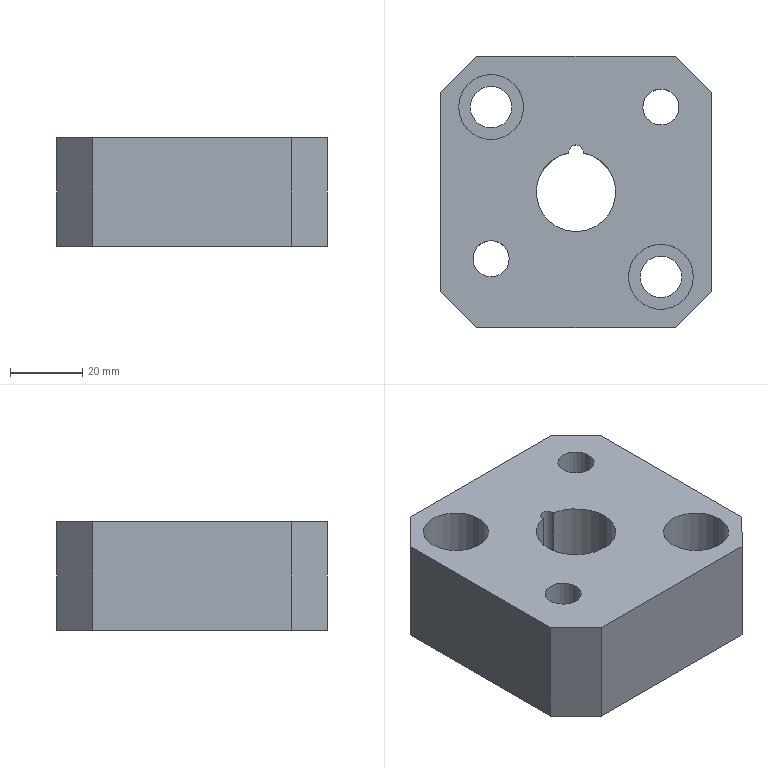Part | NX | features 23 2 | 1 solid | 20 faces | box 75 x 75 x 30 mm | volume 135687 mm3 | plane 12 | cylinder 8 | commonest cylinder face diameters 10.001 x2 11.5 x2 18 x2 4 x1 22 x1
STEP:
#1=CARTESIAN_POINT('',(23.298,10.818,-33.5));
#2=VERTEX_POINT('',#1);
#3=CARTESIAN_POINT('',(19.315,10.818,-33.5));
#4=VERTEX_POINT('',#3);
#5=CARTESIAN_POINT('',(21.306,11.,-33.5));
#6=DIRECTION('',(0.,0.,1.));
#7=DIRECTION('',(1.,0.,0.));
#8=AXIS2_PLACEMENT_3D('',#5,#6,#7);
#9=CIRCLE('',#8,2.);
#10=EDGE_CURVE('',#2,#4,#9,.T.);
#11=ORIENTED_EDGE('',*,*,#10,.T.);
#12=CARTESIAN_POINT('',(21.306,0.,-33.5));
#13=DIRECTION('',(0.,0.,-1.));
#14=DIRECTION('',(-1.,0.,0.));
#15=AXIS2_PLACEMENT_3D('',#12,#13,#14);
#16=CIRCLE('',#15,11.);
#17=EDGE_CURVE('',#2,#4,#16,.T.);
#18=ORIENTED_EDGE('',*,*,#17,.F.);
#19=EDGE_LOOP('',(#11,#18));
#20=FACE_BOUND('',#19,.T.);
#21=CARTESIAN_POINT('',(-7.194,-18.5,-33.5));
#22=VERTEX_POINT('',#21);
#23=CARTESIAN_POINT('',(-2.194,-18.5,-33.5));
#24=DIRECTION('',(0.,0.,-1.));
#25=DIRECTION('',(-1.,0.,0.));
#26=AXIS2_PLACEMENT_3D('',#23,#24,#25);
#27=CIRCLE('',#26,5.);
#28=EDGE_CURVE('',#22,#22,#27,.T.);
#29=ORIENTED_EDGE('',*,*,#28,.F.);
#30=EDGE_LOOP('',(#29));
#31=FACE_BOUND('',#30,.T.);
#32=CARTESIAN_POINT('',(-7.944,23.5,-33.5));
#33=VERTEX_POINT('',#32);
#34=CARTESIAN_POINT('',(-2.194,23.5,-33.5));
#35=DIRECTION('',(0.,0.,-1.));
#36=DIRECTION('',(-1.,0.,0.));
#37=AXIS2_PLACEMENT_3D('',#34,#35,#36);
#38=CIRCLE('',#37,5.75);
#39=EDGE_CURVE('',#33,#33,#38,.T.);
#40=ORIENTED_EDGE('',*,*,#39,.F.);
#41=EDGE_LOOP('',(#40));
#42=FACE_BOUND('',#41,.T.);
#43=CARTESIAN_POINT('',(39.806,23.5,-33.5));
#44=VERTEX_POINT('',#43);
#45=CARTESIAN_POINT('',(44.806,23.5,-33.5));
#46=DIRECTION('',(0.,0.,-1.));
#47=DIRECTION('',(-1.,0.,0.));
#48=AXIS2_PLACEMENT_3D('',#45,#46,#47);
#49=CIRCLE('',#48,5.);
#50=EDGE_CURVE('',#44,#44,#49,.T.);
#51=ORIENTED_EDGE('',*,*,#50,.F.);
#52=EDGE_LOOP('',(#51));
#53=FACE_BOUND('',#52,.T.);
#54=CARTESIAN_POINT('',(39.056,-23.5,-33.5));
#55=VERTEX_POINT('',#54);
#56=CARTESIAN_POINT('',(44.806,-23.5,-33.5));
#57=DIRECTION('',(0.,0.,-1.));
#58=DIRECTION('',(-1.,0.,0.));
#59=AXIS2_PLACEMENT_3D('',#56,#57,#58);
#60=CIRCLE('',#59,5.75);
#61=EDGE_CURVE('',#55,#55,#60,.T.);
#62=ORIENTED_EDGE('',*,*,#61,.F.);
#63=EDGE_LOOP('',(#62));
#64=FACE_BOUND('',#63,.T.);
#65=CARTESIAN_POINT('',(58.806,-27.5,-33.5));
#66=VERTEX_POINT('',#65);
#67=CARTESIAN_POINT('',(58.806,27.5,-33.5));
#68=VERTEX_POINT('',#67);
#69=CARTESIAN_POINT('',(58.806,0.,-33.5));
#70=DIRECTION('',(0.,1.,0.));
#71=VECTOR('',#70,1000.);
#72=LINE('',#69,#71);
#73=EDGE_CURVE('',#66,#68,#72,.T.);
#74=ORIENTED_EDGE('',*,*,#73,.F.);
#75=CARTESIAN_POINT('',(48.806,-37.5,-33.5));
#76=VERTEX_POINT('',#75);
#77=CARTESIAN_POINT('',(55.297,-31.009,-33.5));
#78=DIRECTION('',(-0.7071,-0.7071,0.));
#79=VECTOR('',#78,1000.);
#80=LINE('',#77,#79);
#81=EDGE_CURVE('',#66,#76,#80,.T.);
#82=ORIENTED_EDGE('',*,*,#81,.T.);
#83=CARTESIAN_POINT('',(-6.194,-37.5,-33.5));
#84=VERTEX_POINT('',#83);
#85=CARTESIAN_POINT('',(21.306,-37.5,-33.5));
#86=DIRECTION('',(1.,0.,0.));
#87=VECTOR('',#86,1000.);
#88=LINE('',#85,#87);
#89=EDGE_CURVE('',#84,#76,#88,.T.);
#90=ORIENTED_EDGE('',*,*,#89,.F.);
#91=CARTESIAN_POINT('',(-16.194,-27.5,-33.5));
#92=VERTEX_POINT('',#91);
#93=CARTESIAN_POINT('',(19.741,-63.435,-33.5));
#94=DIRECTION('',(-0.7071,0.7071,0.));
#95=VECTOR('',#94,1000.);
#96=LINE('',#93,#95);
#97=EDGE_CURVE('',#84,#92,#96,.T.);
#98=ORIENTED_EDGE('',*,*,#97,.T.);
#99=CARTESIAN_POINT('',(-16.194,27.5,-33.5));
#100=VERTEX_POINT('',#99);
#101=CARTESIAN_POINT('',(-16.194,0.,-33.5));
#102=DIRECTION('',(0.,-1.,0.));
#103=VECTOR('',#102,1000.);
#104=LINE('',#101,#103);
#105=EDGE_CURVE('',#100,#92,#104,.T.);
#106=ORIENTED_EDGE('',*,*,#105,.F.);
#107=CARTESIAN_POINT('',(-6.194,37.5,-33.5));
#108=VERTEX_POINT('',#107);
#109=CARTESIAN_POINT('',(-14.703,28.991,-33.5));
#110=DIRECTION('',(0.7071,0.7071,0.));
#111=VECTOR('',#110,1000.);
#112=LINE('',#109,#111);
#113=EDGE_CURVE('',#100,#108,#112,.T.);
#114=ORIENTED_EDGE('',*,*,#113,.T.);
#115=CARTESIAN_POINT('',(48.806,37.5,-33.5));
#116=VERTEX_POINT('',#115);
#117=CARTESIAN_POINT('',(21.306,37.5,-33.5));
#118=DIRECTION('',(-1.,0.,0.));
#119=VECTOR('',#118,1000.);
#120=LINE('',#117,#119);
#121=EDGE_CURVE('',#116,#108,#120,.T.);
#122=ORIENTED_EDGE('',*,*,#121,.F.);
#123=CARTESIAN_POINT('',(89.741,-3.435,-33.5));
#124=DIRECTION('',(0.7071,-0.7071,0.));
#125=VECTOR('',#124,1000.);
#126=LINE('',#123,#125);
#127=EDGE_CURVE('',#116,#68,#126,.T.);
#128=ORIENTED_EDGE('',*,*,#127,.T.);
#129=EDGE_LOOP('',(#74,#82,#90,#98,#106,#114,#122,#128));
#130=FACE_BOUND('',#129,.T.);
#131=CARTESIAN_POINT('',(53.733,-34.444,-33.5));
#132=DIRECTION('',(0.,0.,-1.));
#133=DIRECTION('',(-1.,0.,0.));
#134=AXIS2_PLACEMENT_3D('',#131,#132,#133);
#135=PLANE('',#134);
#136=ADVANCED_FACE('',(#20,#31,#42,#53,#64,#130),#135,.T.);
#137=CARTESIAN_POINT('',(19.315,10.818,-3.5));
#138=VERTEX_POINT('',#137);
#139=CARTESIAN_POINT('',(23.298,10.818,-3.5));
#140=VERTEX_POINT('',#139);
#141=CARTESIAN_POINT('',(21.306,0.,-3.5));
#142=DIRECTION('',(0.,0.,1.));
#143=DIRECTION('',(-1.,0.,0.));
#144=AXIS2_PLACEMENT_3D('',#141,#142,#143);
#145=CIRCLE('',#144,11.);
#146=EDGE_CURVE('',#138,#140,#145,.T.);
#147=ORIENTED_EDGE('',*,*,#146,.F.);
#148=CARTESIAN_POINT('',(21.306,11.,-3.5));
#149=DIRECTION('',(0.,0.,-1.));
#150=DIRECTION('',(-1.,0.,0.));
#151=AXIS2_PLACEMENT_3D('',#148,#149,#150);
#152=CIRCLE('',#151,2.);
#153=EDGE_CURVE('',#138,#140,#152,.T.);
#154=ORIENTED_EDGE('',*,*,#153,.T.);
#155=EDGE_LOOP('',(#147,#154));
#156=FACE_BOUND('',#155,.T.);
#157=CARTESIAN_POINT('',(-11.194,23.5,-3.5));
#158=VERTEX_POINT('',#157);
#159=CARTESIAN_POINT('',(-2.194,23.5,-3.5));
#160=DIRECTION('',(0.,0.,-1.));
#161=DIRECTION('',(-1.,0.,0.));
#162=AXIS2_PLACEMENT_3D('',#159,#160,#161);
#163=CIRCLE('',#162,9.);
#164=EDGE_CURVE('',#158,#158,#163,.T.);
#165=ORIENTED_EDGE('',*,*,#164,.T.);
#166=EDGE_LOOP('',(#165));
#167=FACE_BOUND('',#166,.T.);
#168=CARTESIAN_POINT('',(39.806,23.5,-3.5));
#169=VERTEX_POINT('',#168);
#170=CARTESIAN_POINT('',(44.806,23.5,-3.5));
#171=DIRECTION('',(0.,0.,1.));
#172=DIRECTION('',(-1.,0.,0.));
#173=AXIS2_PLACEMENT_3D('',#170,#171,#172);
#174=CIRCLE('',#173,5.);
#175=EDGE_CURVE('',#169,#169,#174,.T.);
#176=ORIENTED_EDGE('',*,*,#175,.F.);
#177=EDGE_LOOP('',(#176));
#178=FACE_BOUND('',#177,.T.);
#179=CARTESIAN_POINT('',(48.806,-37.5,-3.5));
#180=VERTEX_POINT('',#179);
#181=CARTESIAN_POINT('',(-6.194,-37.5,-3.5));
#182=VERTEX_POINT('',#181);
#183=CARTESIAN_POINT('',(21.306,-37.5,-3.5));
#184=DIRECTION('',(-1.,0.,0.));
#185=VECTOR('',#184,1000.);
#186=LINE('',#183,#185);
#187=EDGE_CURVE('',#180,#182,#186,.T.);
#188=ORIENTED_EDGE('',*,*,#187,.F.);
#189=CARTESIAN_POINT('',(58.806,-27.5,-3.5));
#190=VERTEX_POINT('',#189);
#191=CARTESIAN_POINT('',(64.18,-22.126,-3.5));
#192=DIRECTION('',(0.7071,0.7071,0.));
#193=VECTOR('',#192,1000.);
#194=LINE('',#191,#193);
#195=EDGE_CURVE('',#180,#190,#194,.T.);
#196=ORIENTED_EDGE('',*,*,#195,.T.);
#197=CARTESIAN_POINT('',(58.806,27.5,-3.5));
#198=VERTEX_POINT('',#197);
#199=CARTESIAN_POINT('',(58.806,0.,-3.5));
#200=DIRECTION('',(0.,-1.,0.));
#201=VECTOR('',#200,1000.);
#202=LINE('',#199,#201);
#203=EDGE_CURVE('',#198,#190,#202,.T.);
#204=ORIENTED_EDGE('',*,*,#203,.F.);
#205=CARTESIAN_POINT('',(48.806,37.5,-3.5));
#206=VERTEX_POINT('',#205);
#207=CARTESIAN_POINT('',(41.505,44.802,-3.5));
#208=DIRECTION('',(-0.7071,0.7071,0.));
#209=VECTOR('',#208,1000.);
#210=LINE('',#207,#209);
#211=EDGE_CURVE('',#198,#206,#210,.T.);
#212=ORIENTED_EDGE('',*,*,#211,.T.);
#213=CARTESIAN_POINT('',(-6.194,37.5,-3.5));
#214=VERTEX_POINT('',#213);
#215=CARTESIAN_POINT('',(21.306,37.5,-3.5));
#216=DIRECTION('',(1.,0.,0.));
#217=VECTOR('',#216,1000.);
#218=LINE('',#215,#217);
#219=EDGE_CURVE('',#214,#206,#218,.T.);
#220=ORIENTED_EDGE('',*,*,#219,.F.);
#221=CARTESIAN_POINT('',(-16.194,27.5,-3.5));
#222=VERTEX_POINT('',#221);
#223=CARTESIAN_POINT('',(-5.82,37.874,-3.5));
#224=DIRECTION('',(-0.7071,-0.7071,0.));
#225=VECTOR('',#224,1000.);
#226=LINE('',#223,#225);
#227=EDGE_CURVE('',#214,#222,#226,.T.);
#228=ORIENTED_EDGE('',*,*,#227,.T.);
#229=CARTESIAN_POINT('',(-16.194,-27.5,-3.5));
#230=VERTEX_POINT('',#229);
#231=CARTESIAN_POINT('',(-16.194,0.,-3.5));
#232=DIRECTION('',(0.,1.,0.));
#233=VECTOR('',#232,1000.);
#234=LINE('',#231,#233);
#235=EDGE_CURVE('',#230,#222,#234,.T.);
#236=ORIENTED_EDGE('',*,*,#235,.F.);
#237=CARTESIAN_POINT('',(-28.495,-15.198,-3.5));
#238=DIRECTION('',(0.7071,-0.7071,0.));
#239=VECTOR('',#238,1000.);
#240=LINE('',#237,#239);
#241=EDGE_CURVE('',#230,#182,#240,.T.);
#242=ORIENTED_EDGE('',*,*,#241,.T.);
#243=EDGE_LOOP('',(#188,#196,#204,#212,#220,#228,#236,#242));
#244=FACE_BOUND('',#243,.T.);
#245=CARTESIAN_POINT('',(35.806,-23.5,-3.5));
#246=VERTEX_POINT('',#245);
#247=CARTESIAN_POINT('',(44.806,-23.5,-3.5));
#248=DIRECTION('',(0.,0.,-1.));
#249=DIRECTION('',(-1.,0.,0.));
#250=AXIS2_PLACEMENT_3D('',#247,#248,#249);
#251=CIRCLE('',#250,9.);
#252=EDGE_CURVE('',#246,#246,#251,.T.);
#253=ORIENTED_EDGE('',*,*,#252,.T.);
#254=EDGE_LOOP('',(#253));
#255=FACE_BOUND('',#254,.T.);
#256=CARTESIAN_POINT('',(-7.194,-18.5,-3.5));
#257=VERTEX_POINT('',#256);
#258=CARTESIAN_POINT('',(-2.194,-18.5,-3.5));
#259=DIRECTION('',(0.,0.,1.));
#260=DIRECTION('',(-1.,0.,0.));
#261=AXIS2_PLACEMENT_3D('',#258,#259,#260);
#262=CIRCLE('',#261,5.);
#263=EDGE_CURVE('',#257,#257,#262,.T.);
#264=ORIENTED_EDGE('',*,*,#263,.F.);
#265=EDGE_LOOP('',(#264));
#266=FACE_BOUND('',#265,.T.);
#267=CARTESIAN_POINT('',(14.378,22.675,-3.5));
#268=DIRECTION('',(0.,0.,-1.));
#269=DIRECTION('',(-1.,0.,0.));
#270=AXIS2_PLACEMENT_3D('',#267,#268,#269);
#271=PLANE('',#270);
#272=ADVANCED_FACE('',(#156,#167,#178,#244,#255,#266),#271,.F.);
#273=ORIENTED_EDGE('',*,*,#89,.T.);
#274=CARTESIAN_POINT('',(48.806,-37.5,-23.5));
#275=DIRECTION('',(0.,0.,1.));
#276=VECTOR('',#275,1000.);
#277=LINE('',#274,#276);
#278=EDGE_CURVE('',#76,#180,#277,.T.);
#279=ORIENTED_EDGE('',*,*,#278,.T.);
#280=ORIENTED_EDGE('',*,*,#187,.T.);
#281=CARTESIAN_POINT('',(-6.194,-37.5,-23.5));
#282=DIRECTION('',(0.,0.,-1.));
#283=VECTOR('',#282,1000.);
#284=LINE('',#281,#283);
#285=EDGE_CURVE('',#182,#84,#284,.T.);
#286=ORIENTED_EDGE('',*,*,#285,.T.);
#287=EDGE_LOOP('',(#273,#279,#280,#286));
#288=FACE_BOUND('',#287,.T.);
#289=CARTESIAN_POINT('',(21.306,-37.5,-23.5));
#290=DIRECTION('',(0.,-1.,0.));
#291=DIRECTION('',(0.,0.,-1.));
#292=AXIS2_PLACEMENT_3D('',#289,#290,#291);
#293=PLANE('',#292);
#294=ADVANCED_FACE('',(#288),#293,.T.);
#295=ORIENTED_EDGE('',*,*,#235,.T.);
#296=CARTESIAN_POINT('',(-16.194,27.5,-23.5));
#297=DIRECTION('',(0.,0.,-1.));
#298=VECTOR('',#297,1000.);
#299=LINE('',#296,#298);
#300=EDGE_CURVE('',#222,#100,#299,.T.);
#301=ORIENTED_EDGE('',*,*,#300,.T.);
#302=ORIENTED_EDGE('',*,*,#105,.T.);
#303=CARTESIAN_POINT('',(-16.194,-27.5,-23.5));
#304=DIRECTION('',(0.,0.,1.));
#305=VECTOR('',#304,1000.);
#306=LINE('',#303,#305);
#307=EDGE_CURVE('',#92,#230,#306,.T.);
#308=ORIENTED_EDGE('',*,*,#307,.T.);
#309=EDGE_LOOP('',(#295,#301,#302,#308));
#310=FACE_BOUND('',#309,.T.);
#311=CARTESIAN_POINT('',(-16.194,0.,-23.5));
#312=DIRECTION('',(-1.,0.,0.));
#313=DIRECTION('',(0.,0.,1.));
#314=AXIS2_PLACEMENT_3D('',#311,#312,#313);
#315=PLANE('',#314);
#316=ADVANCED_FACE('',(#310),#315,.T.);
#317=ORIENTED_EDGE('',*,*,#219,.T.);
#318=CARTESIAN_POINT('',(48.806,37.5,-23.5));
#319=DIRECTION('',(0.,0.,-1.));
#320=VECTOR('',#319,1000.);
#321=LINE('',#318,#320);
#322=EDGE_CURVE('',#206,#116,#321,.T.);
#323=ORIENTED_EDGE('',*,*,#322,.T.);
#324=ORIENTED_EDGE('',*,*,#121,.T.);
#325=CARTESIAN_POINT('',(-6.194,37.5,-23.5));
#326=DIRECTION('',(0.,0.,1.));
#327=VECTOR('',#326,1000.);
#328=LINE('',#325,#327);
#329=EDGE_CURVE('',#108,#214,#328,.T.);
#330=ORIENTED_EDGE('',*,*,#329,.T.);
#331=EDGE_LOOP('',(#317,#323,#324,#330));
#332=FACE_BOUND('',#331,.T.);
#333=CARTESIAN_POINT('',(21.306,37.5,-23.5));
#334=DIRECTION('',(0.,1.,0.));
#335=DIRECTION('',(0.,0.,1.));
#336=AXIS2_PLACEMENT_3D('',#333,#334,#335);
#337=PLANE('',#336);
#338=ADVANCED_FACE('',(#332),#337,.T.);
#339=ORIENTED_EDGE('',*,*,#203,.T.);
#340=CARTESIAN_POINT('',(58.806,-27.5,-23.5));
#341=DIRECTION('',(0.,0.,-1.));
#342=VECTOR('',#341,1000.);
#343=LINE('',#340,#342);
#344=EDGE_CURVE('',#190,#66,#343,.T.);
#345=ORIENTED_EDGE('',*,*,#344,.T.);
#346=ORIENTED_EDGE('',*,*,#73,.T.);
#347=CARTESIAN_POINT('',(58.806,27.5,-23.5));
#348=DIRECTION('',(0.,0.,1.));
#349=VECTOR('',#348,1000.);
#350=LINE('',#347,#349);
#351=EDGE_CURVE('',#68,#198,#350,.T.);
#352=ORIENTED_EDGE('',*,*,#351,.T.);
#353=EDGE_LOOP('',(#339,#345,#346,#352));
#354=FACE_BOUND('',#353,.T.);
#355=CARTESIAN_POINT('',(58.806,0.,-23.5));
#356=DIRECTION('',(1.,0.,0.));
#357=DIRECTION('',(0.,0.,-1.));
#358=AXIS2_PLACEMENT_3D('',#355,#356,#357);
#359=PLANE('',#358);
#360=ADVANCED_FACE('',(#354),#359,.T.);
#361=ORIENTED_EDGE('',*,*,#61,.T.);
#362=EDGE_LOOP('',(#361));
#363=FACE_BOUND('',#362,.T.);
#364=CARTESIAN_POINT('',(39.056,-23.5,-18.5));
#365=VERTEX_POINT('',#364);
#366=CARTESIAN_POINT('',(44.806,-23.5,-18.5));
#367=DIRECTION('',(0.,0.,-1.));
#368=DIRECTION('',(-1.,0.,0.));
#369=AXIS2_PLACEMENT_3D('',#366,#367,#368);
#370=CIRCLE('',#369,5.75);
#371=EDGE_CURVE('',#365,#365,#370,.T.);
#372=ORIENTED_EDGE('',*,*,#371,.F.);
#373=EDGE_LOOP('',(#372));
#374=FACE_BOUND('',#373,.T.);
#375=CARTESIAN_POINT('',(44.806,-23.5,-1.5));
#376=DIRECTION('',(0.,0.,-1.));
#377=DIRECTION('',(1.,0.,0.));
#378=AXIS2_PLACEMENT_3D('',#375,#376,#377);
#379=CYLINDRICAL_SURFACE('',#378,5.75);
#380=ADVANCED_FACE('',(#363,#374),#379,.F.);
#381=ORIENTED_EDGE('',*,*,#371,.T.);
#382=EDGE_LOOP('',(#381));
#383=FACE_BOUND('',#382,.T.);
#384=CARTESIAN_POINT('',(35.806,-23.5,-18.5));
#385=VERTEX_POINT('',#384);
#386=CARTESIAN_POINT('',(44.806,-23.5,-18.5));
#387=DIRECTION('',(0.,0.,-1.));
#388=DIRECTION('',(-1.,0.,0.));
#389=AXIS2_PLACEMENT_3D('',#386,#387,#388);
#390=CIRCLE('',#389,9.);
#391=EDGE_CURVE('',#385,#385,#390,.T.);
#392=ORIENTED_EDGE('',*,*,#391,.F.);
#393=EDGE_LOOP('',(#392));
#394=FACE_BOUND('',#393,.T.);
#395=CARTESIAN_POINT('',(44.806,-23.5,-18.5));
#396=DIRECTION('',(0.,0.,-1.));
#397=DIRECTION('',(-1.,0.,0.));
#398=AXIS2_PLACEMENT_3D('',#395,#396,#397);
#399=PLANE('',#398);
#400=ADVANCED_FACE('',(#383,#394),#399,.F.);
#401=ORIENTED_EDGE('',*,*,#391,.T.);
#402=EDGE_LOOP('',(#401));
#403=FACE_BOUND('',#402,.T.);
#404=ORIENTED_EDGE('',*,*,#252,.F.);
#405=EDGE_LOOP('',(#404));
#406=FACE_BOUND('',#405,.T.);
#407=CARTESIAN_POINT('',(44.806,-23.5,-3.5));
#408=DIRECTION('',(0.,0.,-1.));
#409=DIRECTION('',(1.,0.,0.));
#410=AXIS2_PLACEMENT_3D('',#407,#408,#409);
#411=CYLINDRICAL_SURFACE('',#410,9.);
#412=ADVANCED_FACE('',(#403,#406),#411,.F.);
#413=ORIENTED_EDGE('',*,*,#175,.T.);
#414=EDGE_LOOP('',(#413));
#415=FACE_BOUND('',#414,.T.);
#416=ORIENTED_EDGE('',*,*,#50,.T.);
#417=EDGE_LOOP('',(#416));
#418=FACE_BOUND('',#417,.T.);
#419=CARTESIAN_POINT('',(44.806,23.5,198.5));
#420=DIRECTION('',(0.,0.,-1.));
#421=DIRECTION('',(-1.,0.,0.));
#422=AXIS2_PLACEMENT_3D('',#419,#420,#421);
#423=CYLINDRICAL_SURFACE('',#422,5.);
#424=ADVANCED_FACE('',(#415,#418),#423,.F.);
#425=ORIENTED_EDGE('',*,*,#39,.T.);
#426=EDGE_LOOP('',(#425));
#427=FACE_BOUND('',#426,.T.);
#428=CARTESIAN_POINT('',(-7.944,23.5,-18.5));
#429=VERTEX_POINT('',#428);
#430=CARTESIAN_POINT('',(-2.194,23.5,-18.5));
#431=DIRECTION('',(0.,0.,-1.));
#432=DIRECTION('',(-1.,0.,0.));
#433=AXIS2_PLACEMENT_3D('',#430,#431,#432);
#434=CIRCLE('',#433,5.75);
#435=EDGE_CURVE('',#429,#429,#434,.T.);
#436=ORIENTED_EDGE('',*,*,#435,.F.);
#437=EDGE_LOOP('',(#436));
#438=FACE_BOUND('',#437,.T.);
#439=CARTESIAN_POINT('',(-2.194,23.5,-1.5));
#440=DIRECTION('',(0.,0.,-1.));
#441=DIRECTION('',(1.,0.,0.));
#442=AXIS2_PLACEMENT_3D('',#439,#440,#441);
#443=CYLINDRICAL_SURFACE('',#442,5.75);
#444=ADVANCED_FACE('',(#427,#438),#443,.F.);
#445=ORIENTED_EDGE('',*,*,#435,.T.);
#446=EDGE_LOOP('',(#445));
#447=FACE_BOUND('',#446,.T.);
#448=CARTESIAN_POINT('',(-11.194,23.5,-18.5));
#449=VERTEX_POINT('',#448);
#450=CARTESIAN_POINT('',(-2.194,23.5,-18.5));
#451=DIRECTION('',(0.,0.,-1.));
#452=DIRECTION('',(-1.,0.,0.));
#453=AXIS2_PLACEMENT_3D('',#450,#451,#452);
#454=CIRCLE('',#453,9.);
#455=EDGE_CURVE('',#449,#449,#454,.T.);
#456=ORIENTED_EDGE('',*,*,#455,.F.);
#457=EDGE_LOOP('',(#456));
#458=FACE_BOUND('',#457,.T.);
#459=CARTESIAN_POINT('',(-2.194,23.5,-18.5));
#460=DIRECTION('',(0.,0.,-1.));
#461=DIRECTION('',(-1.,0.,0.));
#462=AXIS2_PLACEMENT_3D('',#459,#460,#461);
#463=PLANE('',#462);
#464=ADVANCED_FACE('',(#447,#458),#463,.F.);
#465=ORIENTED_EDGE('',*,*,#455,.T.);
#466=EDGE_LOOP('',(#465));
#467=FACE_BOUND('',#466,.T.);
#468=ORIENTED_EDGE('',*,*,#164,.F.);
#469=EDGE_LOOP('',(#468));
#470=FACE_BOUND('',#469,.T.);
#471=CARTESIAN_POINT('',(-2.194,23.5,-3.5));
#472=DIRECTION('',(0.,0.,-1.));
#473=DIRECTION('',(1.,0.,0.));
#474=AXIS2_PLACEMENT_3D('',#471,#472,#473);
#475=CYLINDRICAL_SURFACE('',#474,9.);
#476=ADVANCED_FACE('',(#467,#470),#475,.F.);
#477=ORIENTED_EDGE('',*,*,#263,.T.);
#478=EDGE_LOOP('',(#477));
#479=FACE_BOUND('',#478,.T.);
#480=ORIENTED_EDGE('',*,*,#28,.T.);
#481=EDGE_LOOP('',(#480));
#482=FACE_BOUND('',#481,.T.);
#483=CARTESIAN_POINT('',(-2.194,-18.5,198.5));
#484=DIRECTION('',(0.,0.,-1.));
#485=DIRECTION('',(-1.,0.,0.));
#486=AXIS2_PLACEMENT_3D('',#483,#484,#485);
#487=CYLINDRICAL_SURFACE('',#486,5.);
#488=ADVANCED_FACE('',(#479,#482),#487,.F.);
#489=ORIENTED_EDGE('',*,*,#81,.F.);
#490=ORIENTED_EDGE('',*,*,#344,.F.);
#491=ORIENTED_EDGE('',*,*,#195,.F.);
#492=ORIENTED_EDGE('',*,*,#278,.F.);
#493=EDGE_LOOP('',(#489,#490,#491,#492));
#494=FACE_BOUND('',#493,.T.);
#495=CARTESIAN_POINT('',(53.806,-32.5,-23.5));
#496=DIRECTION('',(-0.7071,0.7071,0.));
#497=DIRECTION('',(0.,0.,1.));
#498=AXIS2_PLACEMENT_3D('',#495,#496,#497);
#499=PLANE('',#498);
#500=ADVANCED_FACE('',(#494),#499,.F.);
#501=ORIENTED_EDGE('',*,*,#127,.F.);
#502=ORIENTED_EDGE('',*,*,#322,.F.);
#503=ORIENTED_EDGE('',*,*,#211,.F.);
#504=ORIENTED_EDGE('',*,*,#351,.F.);
#505=EDGE_LOOP('',(#501,#502,#503,#504));
#506=FACE_BOUND('',#505,.T.);
#507=CARTESIAN_POINT('',(58.806,27.5,-23.5));
#508=DIRECTION('',(-0.7071,-0.7071,0.));
#509=DIRECTION('',(0.,0.,1.));
#510=AXIS2_PLACEMENT_3D('',#507,#508,#509);
#511=PLANE('',#510);
#512=ADVANCED_FACE('',(#506),#511,.F.);
#513=ORIENTED_EDGE('',*,*,#113,.F.);
#514=ORIENTED_EDGE('',*,*,#300,.F.);
#515=ORIENTED_EDGE('',*,*,#227,.F.);
#516=ORIENTED_EDGE('',*,*,#329,.F.);
#517=EDGE_LOOP('',(#513,#514,#515,#516));
#518=FACE_BOUND('',#517,.T.);
#519=CARTESIAN_POINT('',(-11.194,32.5,-23.5));
#520=DIRECTION('',(0.7071,-0.7071,0.));
#521=DIRECTION('',(0.,0.,1.));
#522=AXIS2_PLACEMENT_3D('',#519,#520,#521);
#523=PLANE('',#522);
#524=ADVANCED_FACE('',(#518),#523,.F.);
#525=ORIENTED_EDGE('',*,*,#97,.F.);
#526=ORIENTED_EDGE('',*,*,#285,.F.);
#527=ORIENTED_EDGE('',*,*,#241,.F.);
#528=ORIENTED_EDGE('',*,*,#307,.F.);
#529=EDGE_LOOP('',(#525,#526,#527,#528));
#530=FACE_BOUND('',#529,.T.);
#531=CARTESIAN_POINT('',(-16.194,-27.5,-23.5));
#532=DIRECTION('',(0.7071,0.7071,0.));
#533=DIRECTION('',(0.,0.,1.));
#534=AXIS2_PLACEMENT_3D('',#531,#532,#533);
#535=PLANE('',#534);
#536=ADVANCED_FACE('',(#530),#535,.F.);
#537=ORIENTED_EDGE('',*,*,#17,.T.);
#538=CARTESIAN_POINT('',(19.315,10.818,16.5));
#539=DIRECTION('',(0.,0.,1.));
#540=VECTOR('',#539,1000.);
#541=LINE('',#538,#540);
#542=EDGE_CURVE('',#4,#138,#541,.T.);
#543=ORIENTED_EDGE('',*,*,#542,.T.);
#544=ORIENTED_EDGE('',*,*,#146,.T.);
#545=CARTESIAN_POINT('',(23.298,10.818,16.5));
#546=DIRECTION('',(0.,0.,-1.));
#547=VECTOR('',#546,1000.);
#548=LINE('',#545,#547);
#549=EDGE_CURVE('',#140,#2,#548,.T.);
#550=ORIENTED_EDGE('',*,*,#549,.T.);
#551=EDGE_LOOP('',(#537,#543,#544,#550));
#552=FACE_BOUND('',#551,.T.);
#553=CARTESIAN_POINT('',(21.306,0.,-18.5));
#554=DIRECTION('',(0.,0.,1.));
#555=DIRECTION('',(1.,0.,0.));
#556=AXIS2_PLACEMENT_3D('',#553,#554,#555);
#557=CYLINDRICAL_SURFACE('',#556,11.);
#558=ADVANCED_FACE('',(#552),#557,.F.);
#559=ORIENTED_EDGE('',*,*,#10,.F.);
#560=ORIENTED_EDGE('',*,*,#549,.F.);
#561=ORIENTED_EDGE('',*,*,#153,.F.);
#562=ORIENTED_EDGE('',*,*,#542,.F.);
#563=EDGE_LOOP('',(#559,#560,#561,#562));
#564=FACE_BOUND('',#563,.T.);
#565=CARTESIAN_POINT('',(21.306,11.,-33.5));
#566=DIRECTION('',(0.,0.,1.));
#567=DIRECTION('',(-1.,0.,0.));
#568=AXIS2_PLACEMENT_3D('',#565,#566,#567);
#569=CYLINDRICAL_SURFACE('',#568,2.);
#570=ADVANCED_FACE('',(#564),#569,.F.);
#571=CLOSED_SHELL('',(#136,#272,#294,#316,#338,#360,#380,#400,#412,#424,#444,#464,#476,#488,#500,#512,#524,#536,#558,#570));
#572=MANIFOLD_SOLID_BREP('',#571);
#573=(LENGTH_UNIT()NAMED_UNIT(*)SI_UNIT(.MILLI.,.METRE.));
#574=UNCERTAINTY_MEASURE_WITH_UNIT(LENGTH_MEASURE(0.00001),#573,'','');
#575=(NAMED_UNIT(*)PLANE_ANGLE_UNIT()SI_UNIT($,.RADIAN.));
#576=(NAMED_UNIT(*)SI_UNIT($,.STERADIAN.)SOLID_ANGLE_UNIT());
#577=(GEOMETRIC_REPRESENTATION_CONTEXT(3)GLOBAL_UNCERTAINTY_ASSIGNED_CONTEXT((#574))GLOBAL_UNIT_ASSIGNED_CONTEXT((#573,#575,#576))REPRESENTATION_CONTEXT('',''));
#578=ADVANCED_BREP_SHAPE_REPRESENTATION('',(#572),#577);